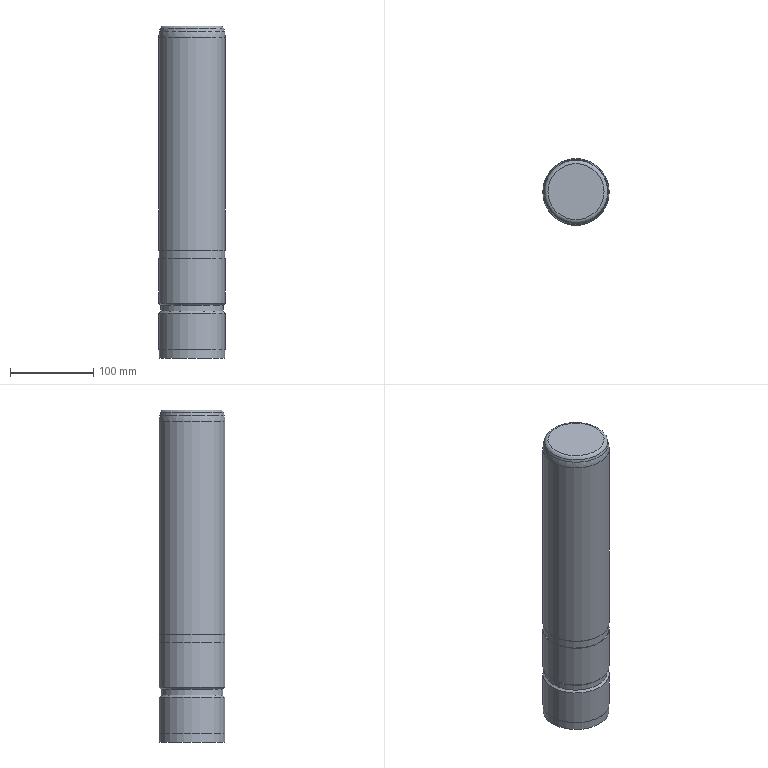Part | NX | features solid 2 | 1 solid | 16 faces | box 80 x 80 x 400 mm | volume 1998956 mm3 | cylinder 6 | plane 5 | cone 3 | torus 2 | commonest cylinder face diameters 80 x3 75 x1 79 x1 79.5 x1
STEP:
#1=CARTESIAN_POINT('',(-1207.5,500.,-181.5));
#2=VERTEX_POINT('',#1);
#3=CARTESIAN_POINT('',(-1170.,500.,-181.5));
#4=DIRECTION('',(0.,0.,1.));
#5=DIRECTION('',(-1.,0.,0.));
#6=AXIS2_PLACEMENT_3D('',#3,#4,#5);
#7=CIRCLE('',#6,37.5);
#8=EDGE_CURVE('',#2,#2,#7,.T.);
#9=ORIENTED_EDGE('',*,*,#8,.T.);
#10=EDGE_LOOP('',(#9));
#11=FACE_BOUND('',#10,.T.);
#12=CARTESIAN_POINT('',(-1130.,500.,-179.));
#13=VERTEX_POINT('',#12);
#14=CARTESIAN_POINT('',(-1170.,500.,-179.));
#15=DIRECTION('',(0.,0.,-1.));
#16=DIRECTION('',(1.,0.,0.));
#17=AXIS2_PLACEMENT_3D('',#14,#15,#16);
#18=CIRCLE('',#17,40.);
#19=EDGE_CURVE('',#13,#13,#18,.T.);
#20=ORIENTED_EDGE('',*,*,#19,.T.);
#21=EDGE_LOOP('',(#20));
#22=FACE_BOUND('',#21,.T.);
#23=CARTESIAN_POINT('',(-1170.,500.,-181.5));
#24=DIRECTION('',(0.,0.,1.));
#25=DIRECTION('',(1.,0.,0.));
#26=AXIS2_PLACEMENT_3D('',#23,#24,#25);
#27=CONICAL_SURFACE('',#26,37.5,0.7854);
#28=ADVANCED_FACE('',(#11,#22),#27,.T.);
#29=ORIENTED_EDGE('',*,*,#8,.F.);
#30=EDGE_LOOP('',(#29));
#31=FACE_BOUND('',#30,.T.);
#32=CARTESIAN_POINT('',(-1207.5,500.,-188.5));
#33=VERTEX_POINT('',#32);
#34=CARTESIAN_POINT('',(-1170.,500.,-188.5));
#35=DIRECTION('',(0.,0.,1.));
#36=DIRECTION('',(-1.,0.,0.));
#37=AXIS2_PLACEMENT_3D('',#34,#35,#36);
#38=CIRCLE('',#37,37.5);
#39=EDGE_CURVE('',#33,#33,#38,.T.);
#40=ORIENTED_EDGE('',*,*,#39,.T.);
#41=EDGE_LOOP('',(#40));
#42=FACE_BOUND('',#41,.T.);
#43=CARTESIAN_POINT('',(-1170.,500.,-188.5));
#44=DIRECTION('',(0.,0.,1.));
#45=DIRECTION('',(1.,0.,0.));
#46=AXIS2_PLACEMENT_3D('',#43,#44,#45);
#47=CYLINDRICAL_SURFACE('',#46,37.5);
#48=ADVANCED_FACE('',(#31,#42),#47,.T.);
#49=CARTESIAN_POINT('',(-1130.5,500.,-125.));
#50=VERTEX_POINT('',#49);
#51=CARTESIAN_POINT('',(-1170.,500.,-125.));
#52=DIRECTION('',(0.,0.,-1.));
#53=DIRECTION('',(1.,0.,0.));
#54=AXIS2_PLACEMENT_3D('',#51,#52,#53);
#55=CIRCLE('',#54,39.5);
#56=EDGE_CURVE('',#50,#50,#55,.T.);
#57=ORIENTED_EDGE('',*,*,#56,.T.);
#58=EDGE_LOOP('',(#57));
#59=FACE_BOUND('',#58,.T.);
#60=CARTESIAN_POINT('',(-1210.,500.,-125.));
#61=VERTEX_POINT('',#60);
#62=CARTESIAN_POINT('',(-1170.,500.,-125.));
#63=DIRECTION('',(0.,0.,1.));
#64=DIRECTION('',(-1.,0.,0.));
#65=AXIS2_PLACEMENT_3D('',#62,#63,#64);
#66=CIRCLE('',#65,40.);
#67=EDGE_CURVE('',#61,#61,#66,.T.);
#68=ORIENTED_EDGE('',*,*,#67,.T.);
#69=EDGE_LOOP('',(#68));
#70=FACE_BOUND('',#69,.T.);
#71=CARTESIAN_POINT('',(-1170.,500.,-125.));
#72=DIRECTION('',(0.,0.,1.));
#73=DIRECTION('',(1.,0.,0.));
#74=AXIS2_PLACEMENT_3D('',#71,#72,#73);
#75=PLANE('',#74);
#76=ADVANCED_FACE('',(#59,#70),#75,.T.);
#77=ORIENTED_EDGE('',*,*,#67,.F.);
#78=EDGE_LOOP('',(#77));
#79=FACE_BOUND('',#78,.T.);
#80=ORIENTED_EDGE('',*,*,#19,.F.);
#81=EDGE_LOOP('',(#80));
#82=FACE_BOUND('',#81,.T.);
#83=CARTESIAN_POINT('',(-1170.,500.,-179.));
#84=DIRECTION('',(0.,0.,1.));
#85=DIRECTION('',(1.,0.,0.));
#86=AXIS2_PLACEMENT_3D('',#83,#84,#85);
#87=CYLINDRICAL_SURFACE('',#86,40.);
#88=ADVANCED_FACE('',(#79,#82),#87,.T.);
#89=CARTESIAN_POINT('',(-1209.5,500.,-115.));
#90=VERTEX_POINT('',#89);
#91=CARTESIAN_POINT('',(-1170.,500.,-115.));
#92=DIRECTION('',(0.,0.,1.));
#93=DIRECTION('',(-1.,0.,0.));
#94=AXIS2_PLACEMENT_3D('',#91,#92,#93);
#95=CIRCLE('',#94,39.5);
#96=EDGE_CURVE('',#90,#90,#95,.T.);
#97=ORIENTED_EDGE('',*,*,#96,.T.);
#98=EDGE_LOOP('',(#97));
#99=FACE_BOUND('',#98,.T.);
#100=CARTESIAN_POINT('',(-1130.,500.,-115.));
#101=VERTEX_POINT('',#100);
#102=CARTESIAN_POINT('',(-1170.,500.,-115.));
#103=DIRECTION('',(0.,0.,-1.));
#104=DIRECTION('',(1.,0.,0.));
#105=AXIS2_PLACEMENT_3D('',#102,#103,#104);
#106=CIRCLE('',#105,40.);
#107=EDGE_CURVE('',#101,#101,#106,.T.);
#108=ORIENTED_EDGE('',*,*,#107,.T.);
#109=EDGE_LOOP('',(#108));
#110=FACE_BOUND('',#109,.T.);
#111=CARTESIAN_POINT('',(-1170.,500.,-115.));
#112=DIRECTION('',(0.,0.,-1.));
#113=DIRECTION('',(-1.,0.,0.));
#114=AXIS2_PLACEMENT_3D('',#111,#112,#113);
#115=PLANE('',#114);
#116=ADVANCED_FACE('',(#99,#110),#115,.T.);
#117=CARTESIAN_POINT('',(-1210.,500.,141.05));
#118=VERTEX_POINT('',#117);
#119=CARTESIAN_POINT('',(-1170.,500.,141.05));
#120=DIRECTION('',(0.,0.,1.));
#121=DIRECTION('',(-1.,0.,0.));
#122=AXIS2_PLACEMENT_3D('',#119,#120,#121);
#123=CIRCLE('',#122,40.);
#124=EDGE_CURVE('',#118,#118,#123,.T.);
#125=ORIENTED_EDGE('',*,*,#124,.F.);
#126=EDGE_LOOP('',(#125));
#127=FACE_BOUND('',#126,.T.);
#128=ORIENTED_EDGE('',*,*,#107,.F.);
#129=EDGE_LOOP('',(#128));
#130=FACE_BOUND('',#129,.T.);
#131=CARTESIAN_POINT('',(-1170.,500.,-115.));
#132=DIRECTION('',(0.,0.,1.));
#133=DIRECTION('',(1.,0.,0.));
#134=AXIS2_PLACEMENT_3D('',#131,#132,#133);
#135=CYLINDRICAL_SURFACE('',#134,40.);
#136=ADVANCED_FACE('',(#127,#130),#135,.T.);
#137=ORIENTED_EDGE('',*,*,#96,.F.);
#138=EDGE_LOOP('',(#137));
#139=FACE_BOUND('',#138,.T.);
#140=ORIENTED_EDGE('',*,*,#56,.F.);
#141=EDGE_LOOP('',(#140));
#142=FACE_BOUND('',#141,.T.);
#143=CARTESIAN_POINT('',(-1170.,500.,-125.));
#144=DIRECTION('',(0.,0.,1.));
#145=DIRECTION('',(1.,0.,0.));
#146=AXIS2_PLACEMENT_3D('',#143,#144,#145);
#147=CYLINDRICAL_SURFACE('',#146,39.5);
#148=ADVANCED_FACE('',(#139,#142),#147,.T.);
#149=CARTESIAN_POINT('',(-1136.132,500.,155.));
#150=VERTEX_POINT('',#149);
#151=CARTESIAN_POINT('',(-1170.,500.,155.));
#152=DIRECTION('',(0.,0.,-1.));
#153=DIRECTION('',(1.,0.,0.));
#154=AXIS2_PLACEMENT_3D('',#151,#152,#153);
#155=CIRCLE('',#154,33.868);
#156=EDGE_CURVE('',#150,#150,#155,.T.);
#157=ORIENTED_EDGE('',*,*,#156,.F.);
#158=EDGE_LOOP('',(#157));
#159=FACE_BOUND('',#158,.T.);
#160=CARTESIAN_POINT('',(-1170.,500.,155.));
#161=DIRECTION('',(0.,0.,1.));
#162=DIRECTION('',(1.,0.,0.));
#163=AXIS2_PLACEMENT_3D('',#160,#161,#162);
#164=PLANE('',#163);
#165=ADVANCED_FACE('',(#159),#164,.T.);
#166=CARTESIAN_POINT('',(-1131.786,500.,151.665));
#167=VERTEX_POINT('',#166);
#168=CARTESIAN_POINT('',(-1170.,500.,151.665));
#169=DIRECTION('',(0.,0.,-1.));
#170=DIRECTION('',(1.,0.,0.));
#171=AXIS2_PLACEMENT_3D('',#168,#169,#170);
#172=CIRCLE('',#171,38.214);
#173=EDGE_CURVE('',#167,#167,#172,.F.);
#174=ORIENTED_EDGE('',*,*,#173,.F.);
#175=EDGE_LOOP('',(#174));
#176=FACE_BOUND('',#175,.T.);
#177=CARTESIAN_POINT('',(-1131.022,500.,148.815));
#178=VERTEX_POINT('',#177);
#179=CARTESIAN_POINT('',(-1170.,500.,148.815));
#180=DIRECTION('',(0.,0.,-1.));
#181=DIRECTION('',(1.,0.,0.));
#182=AXIS2_PLACEMENT_3D('',#179,#180,#181);
#183=CIRCLE('',#182,38.978);
#184=EDGE_CURVE('',#178,#178,#183,.T.);
#185=ORIENTED_EDGE('',*,*,#184,.F.);
#186=EDGE_LOOP('',(#185));
#187=FACE_BOUND('',#186,.T.);
#188=CARTESIAN_POINT('',(-1170.,500.,155.));
#189=DIRECTION('',(0.,0.,-1.));
#190=DIRECTION('',(-1.,0.,0.));
#191=AXIS2_PLACEMENT_3D('',#188,#189,#190);
#192=CONICAL_SURFACE('',#191,37.321,0.2618);
#193=ADVANCED_FACE('',(#176,#187),#192,.T.);
#194=CARTESIAN_POINT('',(-1209.75,500.,-235.));
#195=VERTEX_POINT('',#194);
#196=CARTESIAN_POINT('',(-1170.,500.,-235.));
#197=DIRECTION('',(0.,0.,1.));
#198=DIRECTION('',(-1.,0.,0.));
#199=AXIS2_PLACEMENT_3D('',#196,#197,#198);
#200=CIRCLE('',#199,39.75);
#201=EDGE_CURVE('',#195,#195,#200,.T.);
#202=ORIENTED_EDGE('',*,*,#201,.T.);
#203=EDGE_LOOP('',(#202));
#204=FACE_BOUND('',#203,.T.);
#205=CARTESIAN_POINT('',(-1130.,500.,-235.));
#206=VERTEX_POINT('',#205);
#207=CARTESIAN_POINT('',(-1170.,500.,-235.));
#208=DIRECTION('',(0.,0.,-1.));
#209=DIRECTION('',(1.,0.,0.));
#210=AXIS2_PLACEMENT_3D('',#207,#208,#209);
#211=CIRCLE('',#210,40.);
#212=EDGE_CURVE('',#206,#206,#211,.T.);
#213=ORIENTED_EDGE('',*,*,#212,.T.);
#214=EDGE_LOOP('',(#213));
#215=FACE_BOUND('',#214,.T.);
#216=CARTESIAN_POINT('',(-1170.,500.,-235.));
#217=DIRECTION('',(0.,0.,-1.));
#218=DIRECTION('',(-1.,0.,0.));
#219=AXIS2_PLACEMENT_3D('',#216,#217,#218);
#220=PLANE('',#219);
#221=ADVANCED_FACE('',(#204,#215),#220,.T.);
#222=CARTESIAN_POINT('',(-1130.,500.,-191.));
#223=VERTEX_POINT('',#222);
#224=CARTESIAN_POINT('',(-1170.,500.,-191.));
#225=DIRECTION('',(0.,0.,-1.));
#226=DIRECTION('',(1.,0.,0.));
#227=AXIS2_PLACEMENT_3D('',#224,#225,#226);
#228=CIRCLE('',#227,40.);
#229=EDGE_CURVE('',#223,#223,#228,.T.);
#230=ORIENTED_EDGE('',*,*,#229,.T.);
#231=EDGE_LOOP('',(#230));
#232=FACE_BOUND('',#231,.T.);
#233=ORIENTED_EDGE('',*,*,#212,.F.);
#234=EDGE_LOOP('',(#233));
#235=FACE_BOUND('',#234,.T.);
#236=CARTESIAN_POINT('',(-1170.,500.,-235.));
#237=DIRECTION('',(0.,0.,1.));
#238=DIRECTION('',(1.,0.,0.));
#239=AXIS2_PLACEMENT_3D('',#236,#237,#238);
#240=CYLINDRICAL_SURFACE('',#239,40.);
#241=ADVANCED_FACE('',(#232,#235),#240,.T.);
#242=CARTESIAN_POINT('',(-1130.25,500.,-245.));
#243=VERTEX_POINT('',#242);
#244=CARTESIAN_POINT('',(-1170.,500.,-245.));
#245=DIRECTION('',(0.,0.,-1.));
#246=DIRECTION('',(1.,0.,0.));
#247=AXIS2_PLACEMENT_3D('',#244,#245,#246);
#248=CIRCLE('',#247,39.75);
#249=EDGE_CURVE('',#243,#243,#248,.T.);
#250=ORIENTED_EDGE('',*,*,#249,.T.);
#251=EDGE_LOOP('',(#250));
#252=FACE_BOUND('',#251,.T.);
#253=CARTESIAN_POINT('',(-1170.,500.,-245.));
#254=DIRECTION('',(0.,0.,-1.));
#255=DIRECTION('',(-1.,0.,0.));
#256=AXIS2_PLACEMENT_3D('',#253,#254,#255);
#257=PLANE('',#256);
#258=ADVANCED_FACE('',(#252),#257,.T.);
#259=ORIENTED_EDGE('',*,*,#201,.F.);
#260=EDGE_LOOP('',(#259));
#261=FACE_BOUND('',#260,.T.);
#262=ORIENTED_EDGE('',*,*,#249,.F.);
#263=EDGE_LOOP('',(#262));
#264=FACE_BOUND('',#263,.T.);
#265=CARTESIAN_POINT('',(-1170.,500.,-245.));
#266=DIRECTION('',(0.,0.,1.));
#267=DIRECTION('',(1.,0.,0.));
#268=AXIS2_PLACEMENT_3D('',#265,#266,#267);
#269=CYLINDRICAL_SURFACE('',#268,39.75);
#270=ADVANCED_FACE('',(#261,#264),#269,.T.);
#271=ORIENTED_EDGE('',*,*,#229,.F.);
#272=EDGE_LOOP('',(#271));
#273=FACE_BOUND('',#272,.T.);
#274=ORIENTED_EDGE('',*,*,#39,.F.);
#275=EDGE_LOOP('',(#274));
#276=FACE_BOUND('',#275,.T.);
#277=CARTESIAN_POINT('',(-1170.,500.,-188.5));
#278=DIRECTION('',(0.,0.,-1.));
#279=DIRECTION('',(-1.,0.,0.));
#280=AXIS2_PLACEMENT_3D('',#277,#278,#279);
#281=CONICAL_SURFACE('',#280,37.5,0.7854);
#282=ADVANCED_FACE('',(#273,#276),#281,.T.);
#283=ORIENTED_EDGE('',*,*,#124,.T.);
#284=EDGE_LOOP('',(#283));
#285=FACE_BOUND('',#284,.T.);
#286=ORIENTED_EDGE('',*,*,#184,.T.);
#287=EDGE_LOOP('',(#286));
#288=FACE_BOUND('',#287,.T.);
#289=CARTESIAN_POINT('',(-1170.,500.,141.05));
#290=DIRECTION('',(0.,0.,-1.));
#291=DIRECTION('',(-1.,0.,0.));
#292=AXIS2_PLACEMENT_3D('',#289,#290,#291);
#293=DEGENERATE_TOROIDAL_SURFACE('',#292,10.,30.,.T.);
#294=ADVANCED_FACE('',(#285,#288),#293,.T.);
#295=ORIENTED_EDGE('',*,*,#156,.T.);
#296=EDGE_LOOP('',(#295));
#297=FACE_BOUND('',#296,.T.);
#298=ORIENTED_EDGE('',*,*,#173,.T.);
#299=EDGE_LOOP('',(#298));
#300=FACE_BOUND('',#299,.T.);
#301=CARTESIAN_POINT('',(-1170.,500.,150.5));
#302=DIRECTION('',(0.,0.,1.));
#303=DIRECTION('',(1.,0.,0.));
#304=AXIS2_PLACEMENT_3D('',#301,#302,#303);
#305=TOROIDAL_SURFACE('',#304,33.868,4.5);
#306=ADVANCED_FACE('',(#297,#300),#305,.T.);
#307=CLOSED_SHELL('',(#28,#48,#76,#88,#116,#136,#148,#165,#193,#221,#241,#258,#270,#282,#294,#306));
#308=MANIFOLD_SOLID_BREP('',#307);
#309=(LENGTH_UNIT()NAMED_UNIT(*)SI_UNIT(.MILLI.,.METRE.));
#310=UNCERTAINTY_MEASURE_WITH_UNIT(LENGTH_MEASURE(0.00001),#309,'','');
#311=(NAMED_UNIT(*)PLANE_ANGLE_UNIT()SI_UNIT($,.RADIAN.));
#312=(NAMED_UNIT(*)SI_UNIT($,.STERADIAN.)SOLID_ANGLE_UNIT());
#313=(GEOMETRIC_REPRESENTATION_CONTEXT(3)GLOBAL_UNCERTAINTY_ASSIGNED_CONTEXT((#310))GLOBAL_UNIT_ASSIGNED_CONTEXT((#309,#311,#312))REPRESENTATION_CONTEXT('',''));
#314=ADVANCED_BREP_SHAPE_REPRESENTATION('',(#308),#313);